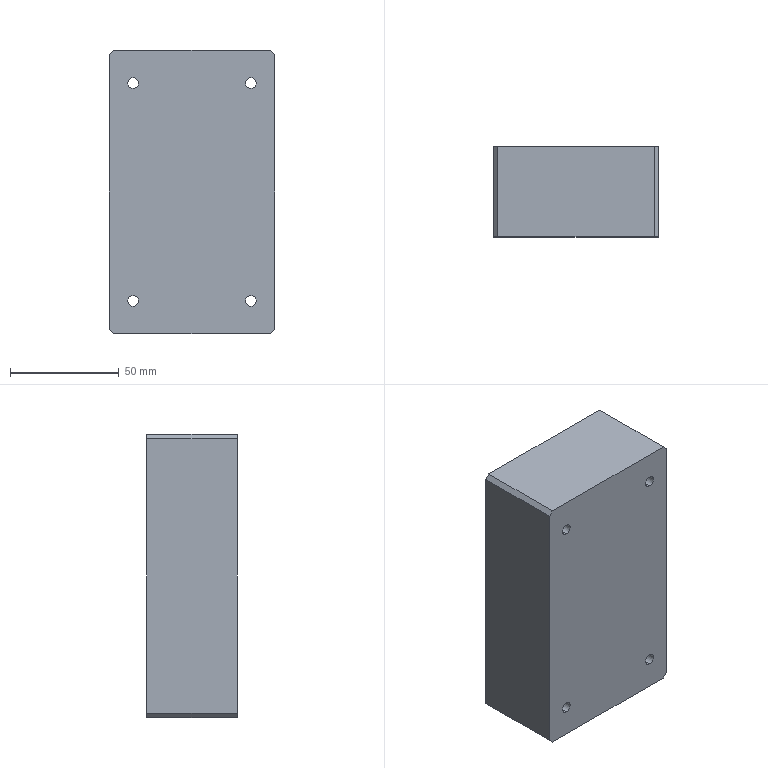Part | SolidWorks | features Chamfer 1, Extrusion 1, HoleWzd 1 | 1 solid | 18 faces | box 76 x 41.5 x 130 mm | volume 406429 mm3 | plane 10 | cylinder 8 | commonest cylinder face diameters 5 x8
STEP:
#1=CARTESIAN_POINT('',(-27.,-20.75,47.5));
#2=VERTEX_POINT('',#1);
#3=CARTESIAN_POINT('',(-27.,-20.75,52.5));
#4=VERTEX_POINT('',#3);
#5=CARTESIAN_POINT('',(-27.,-20.75,50.));
#6=DIRECTION('',(0.,1.,0.));
#7=DIRECTION('',(0.,0.,1.));
#8=AXIS2_PLACEMENT_3D('',#5,#6,#7);
#9=CIRCLE('',#8,2.5);
#10=EDGE_CURVE('',#2,#4,#9,.T.);
#11=ORIENTED_EDGE('',*,*,#10,.F.);
#12=CARTESIAN_POINT('',(-27.,20.75,47.5));
#13=VERTEX_POINT('',#12);
#14=CARTESIAN_POINT('',(-27.,20.75,47.5));
#15=DIRECTION('',(0.,1.,0.));
#16=VECTOR('',#15,1000.);
#17=LINE('',#14,#16);
#18=EDGE_CURVE('',#2,#13,#17,.T.);
#19=ORIENTED_EDGE('',*,*,#18,.T.);
#20=CARTESIAN_POINT('',(-27.,20.75,52.5));
#21=VERTEX_POINT('',#20);
#22=CARTESIAN_POINT('',(-27.,20.75,50.));
#23=DIRECTION('',(0.,1.,0.));
#24=DIRECTION('',(0.,0.,1.));
#25=AXIS2_PLACEMENT_3D('',#22,#23,#24);
#26=CIRCLE('',#25,2.5);
#27=EDGE_CURVE('',#13,#21,#26,.T.);
#28=ORIENTED_EDGE('',*,*,#27,.T.);
#29=CARTESIAN_POINT('',(-27.,20.75,52.5));
#30=DIRECTION('',(0.,1.,0.));
#31=VECTOR('',#30,1000.);
#32=LINE('',#29,#31);
#33=EDGE_CURVE('',#4,#21,#32,.T.);
#34=ORIENTED_EDGE('',*,*,#33,.F.);
#35=EDGE_LOOP('',(#11,#19,#28,#34));
#36=FACE_OUTER_BOUND('',#35,.T.);
#37=CARTESIAN_POINT('',(-27.,20.75,50.));
#38=DIRECTION('',(0.,1.,0.));
#39=DIRECTION('',(0.,0.,1.));
#40=AXIS2_PLACEMENT_3D('',#37,#38,#39);
#41=CYLINDRICAL_SURFACE('',#40,2.5);
#42=ADVANCED_FACE('',(#36),#41,.F.);
#43=CARTESIAN_POINT('',(27.,-20.75,47.5));
#44=VERTEX_POINT('',#43);
#45=CARTESIAN_POINT('',(27.,-20.75,52.5));
#46=VERTEX_POINT('',#45);
#47=CARTESIAN_POINT('',(27.,-20.75,50.));
#48=DIRECTION('',(0.,1.,0.));
#49=DIRECTION('',(0.,0.,1.));
#50=AXIS2_PLACEMENT_3D('',#47,#48,#49);
#51=CIRCLE('',#50,2.5);
#52=EDGE_CURVE('',#44,#46,#51,.T.);
#53=ORIENTED_EDGE('',*,*,#52,.F.);
#54=CARTESIAN_POINT('',(27.,20.75,47.5));
#55=VERTEX_POINT('',#54);
#56=CARTESIAN_POINT('',(27.,20.75,47.5));
#57=DIRECTION('',(0.,1.,0.));
#58=VECTOR('',#57,1000.);
#59=LINE('',#56,#58);
#60=EDGE_CURVE('',#44,#55,#59,.T.);
#61=ORIENTED_EDGE('',*,*,#60,.T.);
#62=CARTESIAN_POINT('',(27.,20.75,52.5));
#63=VERTEX_POINT('',#62);
#64=CARTESIAN_POINT('',(27.,20.75,50.));
#65=DIRECTION('',(0.,1.,0.));
#66=DIRECTION('',(0.,0.,1.));
#67=AXIS2_PLACEMENT_3D('',#64,#65,#66);
#68=CIRCLE('',#67,2.5);
#69=EDGE_CURVE('',#55,#63,#68,.T.);
#70=ORIENTED_EDGE('',*,*,#69,.T.);
#71=CARTESIAN_POINT('',(27.,20.75,52.5));
#72=DIRECTION('',(0.,1.,0.));
#73=VECTOR('',#72,1000.);
#74=LINE('',#71,#73);
#75=EDGE_CURVE('',#46,#63,#74,.T.);
#76=ORIENTED_EDGE('',*,*,#75,.F.);
#77=EDGE_LOOP('',(#53,#61,#70,#76));
#78=FACE_OUTER_BOUND('',#77,.T.);
#79=CARTESIAN_POINT('',(27.,20.75,50.));
#80=DIRECTION('',(0.,1.,0.));
#81=DIRECTION('',(0.,0.,1.));
#82=AXIS2_PLACEMENT_3D('',#79,#80,#81);
#83=CYLINDRICAL_SURFACE('',#82,2.5);
#84=ADVANCED_FACE('',(#78),#83,.F.);
#85=CARTESIAN_POINT('',(27.,-20.75,-52.5));
#86=VERTEX_POINT('',#85);
#87=CARTESIAN_POINT('',(27.,-20.75,-47.5));
#88=VERTEX_POINT('',#87);
#89=CARTESIAN_POINT('',(27.,-20.75,-50.));
#90=DIRECTION('',(0.,1.,0.));
#91=DIRECTION('',(0.,0.,1.));
#92=AXIS2_PLACEMENT_3D('',#89,#90,#91);
#93=CIRCLE('',#92,2.5);
#94=EDGE_CURVE('',#86,#88,#93,.T.);
#95=ORIENTED_EDGE('',*,*,#94,.F.);
#96=CARTESIAN_POINT('',(27.,20.75,-52.5));
#97=VERTEX_POINT('',#96);
#98=CARTESIAN_POINT('',(27.,20.75,-52.5));
#99=DIRECTION('',(0.,1.,0.));
#100=VECTOR('',#99,1000.);
#101=LINE('',#98,#100);
#102=EDGE_CURVE('',#86,#97,#101,.T.);
#103=ORIENTED_EDGE('',*,*,#102,.T.);
#104=CARTESIAN_POINT('',(27.,20.75,-47.5));
#105=VERTEX_POINT('',#104);
#106=CARTESIAN_POINT('',(27.,20.75,-50.));
#107=DIRECTION('',(0.,1.,0.));
#108=DIRECTION('',(0.,0.,1.));
#109=AXIS2_PLACEMENT_3D('',#106,#107,#108);
#110=CIRCLE('',#109,2.5);
#111=EDGE_CURVE('',#97,#105,#110,.T.);
#112=ORIENTED_EDGE('',*,*,#111,.T.);
#113=CARTESIAN_POINT('',(27.,20.75,-47.5));
#114=DIRECTION('',(0.,1.,0.));
#115=VECTOR('',#114,1000.);
#116=LINE('',#113,#115);
#117=EDGE_CURVE('',#88,#105,#116,.T.);
#118=ORIENTED_EDGE('',*,*,#117,.F.);
#119=EDGE_LOOP('',(#95,#103,#112,#118));
#120=FACE_OUTER_BOUND('',#119,.T.);
#121=CARTESIAN_POINT('',(27.,20.75,-50.));
#122=DIRECTION('',(0.,1.,0.));
#123=DIRECTION('',(0.,0.,1.));
#124=AXIS2_PLACEMENT_3D('',#121,#122,#123);
#125=CYLINDRICAL_SURFACE('',#124,2.5);
#126=ADVANCED_FACE('',(#120),#125,.F.);
#127=CARTESIAN_POINT('',(-27.,-20.75,-52.5));
#128=VERTEX_POINT('',#127);
#129=CARTESIAN_POINT('',(-27.,-20.75,-47.5));
#130=VERTEX_POINT('',#129);
#131=CARTESIAN_POINT('',(-27.,-20.75,-50.));
#132=DIRECTION('',(0.,1.,0.));
#133=DIRECTION('',(0.,0.,1.));
#134=AXIS2_PLACEMENT_3D('',#131,#132,#133);
#135=CIRCLE('',#134,2.5);
#136=EDGE_CURVE('',#128,#130,#135,.T.);
#137=ORIENTED_EDGE('',*,*,#136,.F.);
#138=CARTESIAN_POINT('',(-27.,20.75,-52.5));
#139=VERTEX_POINT('',#138);
#140=CARTESIAN_POINT('',(-27.,20.75,-52.5));
#141=DIRECTION('',(0.,1.,0.));
#142=VECTOR('',#141,1000.);
#143=LINE('',#140,#142);
#144=EDGE_CURVE('',#128,#139,#143,.T.);
#145=ORIENTED_EDGE('',*,*,#144,.T.);
#146=CARTESIAN_POINT('',(-27.,20.75,-47.5));
#147=VERTEX_POINT('',#146);
#148=CARTESIAN_POINT('',(-27.,20.75,-50.));
#149=DIRECTION('',(0.,1.,0.));
#150=DIRECTION('',(0.,0.,1.));
#151=AXIS2_PLACEMENT_3D('',#148,#149,#150);
#152=CIRCLE('',#151,2.5);
#153=EDGE_CURVE('',#139,#147,#152,.T.);
#154=ORIENTED_EDGE('',*,*,#153,.T.);
#155=CARTESIAN_POINT('',(-27.,20.75,-47.5));
#156=DIRECTION('',(0.,1.,0.));
#157=VECTOR('',#156,1000.);
#158=LINE('',#155,#157);
#159=EDGE_CURVE('',#130,#147,#158,.T.);
#160=ORIENTED_EDGE('',*,*,#159,.F.);
#161=EDGE_LOOP('',(#137,#145,#154,#160));
#162=FACE_OUTER_BOUND('',#161,.T.);
#163=CARTESIAN_POINT('',(-27.,20.75,-50.));
#164=DIRECTION('',(0.,1.,0.));
#165=DIRECTION('',(0.,0.,1.));
#166=AXIS2_PLACEMENT_3D('',#163,#164,#165);
#167=CYLINDRICAL_SURFACE('',#166,2.5);
#168=ADVANCED_FACE('',(#162),#167,.F.);
#169=CARTESIAN_POINT('',(38.,20.75,63.));
#170=VERTEX_POINT('',#169);
#171=CARTESIAN_POINT('',(38.,20.75,-63.));
#172=VERTEX_POINT('',#171);
#173=CARTESIAN_POINT('',(38.,20.75,65.));
#174=DIRECTION('',(0.,0.,-1.));
#175=VECTOR('',#174,1000.);
#176=LINE('',#173,#175);
#177=EDGE_CURVE('',#170,#172,#176,.T.);
#178=ORIENTED_EDGE('',*,*,#177,.F.);
#179=CARTESIAN_POINT('',(38.,-20.75,63.));
#180=VERTEX_POINT('',#179);
#181=CARTESIAN_POINT('',(38.,-20.75,63.));
#182=DIRECTION('',(0.,-1.,0.));
#183=VECTOR('',#182,1000.);
#184=LINE('',#181,#183);
#185=EDGE_CURVE('',#170,#180,#184,.T.);
#186=ORIENTED_EDGE('',*,*,#185,.T.);
#187=CARTESIAN_POINT('',(38.,-20.75,-63.));
#188=VERTEX_POINT('',#187);
#189=CARTESIAN_POINT('',(38.,-20.75,65.));
#190=DIRECTION('',(0.,0.,-1.));
#191=VECTOR('',#190,1000.);
#192=LINE('',#189,#191);
#193=EDGE_CURVE('',#180,#188,#192,.T.);
#194=ORIENTED_EDGE('',*,*,#193,.T.);
#195=CARTESIAN_POINT('',(38.,20.75,-63.));
#196=DIRECTION('',(0.,1.,0.));
#197=VECTOR('',#196,1000.);
#198=LINE('',#195,#197);
#199=EDGE_CURVE('',#188,#172,#198,.T.);
#200=ORIENTED_EDGE('',*,*,#199,.T.);
#201=EDGE_LOOP('',(#178,#186,#194,#200));
#202=FACE_OUTER_BOUND('',#201,.T.);
#203=CARTESIAN_POINT('',(38.,20.75,65.));
#204=DIRECTION('',(-1.,0.,0.));
#205=DIRECTION('',(0.,0.,1.));
#206=AXIS2_PLACEMENT_3D('',#203,#204,#205);
#207=PLANE('',#206);
#208=ADVANCED_FACE('',(#202),#207,.F.);
#209=CARTESIAN_POINT('',(-27.,20.75,50.));
#210=DIRECTION('',(0.,1.,0.));
#211=DIRECTION('',(0.,0.,1.));
#212=AXIS2_PLACEMENT_3D('',#209,#210,#211);
#213=CIRCLE('',#212,2.5);
#214=EDGE_CURVE('',#21,#13,#213,.T.);
#215=ORIENTED_EDGE('',*,*,#214,.F.);
#216=ORIENTED_EDGE('',*,*,#27,.F.);
#217=EDGE_LOOP('',(#215,#216));
#218=FACE_BOUND('',#217,.T.);
#219=CARTESIAN_POINT('',(27.,20.75,50.));
#220=DIRECTION('',(0.,1.,0.));
#221=DIRECTION('',(0.,0.,1.));
#222=AXIS2_PLACEMENT_3D('',#219,#220,#221);
#223=CIRCLE('',#222,2.5);
#224=EDGE_CURVE('',#63,#55,#223,.T.);
#225=ORIENTED_EDGE('',*,*,#224,.F.);
#226=ORIENTED_EDGE('',*,*,#69,.F.);
#227=EDGE_LOOP('',(#225,#226));
#228=FACE_BOUND('',#227,.T.);
#229=CARTESIAN_POINT('',(27.,20.75,-50.));
#230=DIRECTION('',(0.,1.,0.));
#231=DIRECTION('',(0.,0.,1.));
#232=AXIS2_PLACEMENT_3D('',#229,#230,#231);
#233=CIRCLE('',#232,2.5);
#234=EDGE_CURVE('',#105,#97,#233,.T.);
#235=ORIENTED_EDGE('',*,*,#234,.F.);
#236=ORIENTED_EDGE('',*,*,#111,.F.);
#237=EDGE_LOOP('',(#235,#236));
#238=FACE_BOUND('',#237,.T.);
#239=CARTESIAN_POINT('',(-27.,20.75,-50.));
#240=DIRECTION('',(0.,1.,0.));
#241=DIRECTION('',(0.,0.,1.));
#242=AXIS2_PLACEMENT_3D('',#239,#240,#241);
#243=CIRCLE('',#242,2.5);
#244=EDGE_CURVE('',#147,#139,#243,.T.);
#245=ORIENTED_EDGE('',*,*,#244,.F.);
#246=ORIENTED_EDGE('',*,*,#153,.F.);
#247=EDGE_LOOP('',(#245,#246));
#248=FACE_BOUND('',#247,.T.);
#249=CARTESIAN_POINT('',(-38.,20.75,63.));
#250=VERTEX_POINT('',#249);
#251=CARTESIAN_POINT('',(-38.,20.75,-63.));
#252=VERTEX_POINT('',#251);
#253=CARTESIAN_POINT('',(-38.,20.75,65.));
#254=DIRECTION('',(0.,0.,-1.));
#255=VECTOR('',#254,1000.);
#256=LINE('',#253,#255);
#257=EDGE_CURVE('',#250,#252,#256,.T.);
#258=ORIENTED_EDGE('',*,*,#257,.F.);
#259=CARTESIAN_POINT('',(-36.,20.75,65.));
#260=VERTEX_POINT('',#259);
#261=CARTESIAN_POINT('',(-36.,20.75,65.));
#262=DIRECTION('',(0.7071,0.,0.7071));
#263=VECTOR('',#262,1000.);
#264=LINE('',#261,#263);
#265=EDGE_CURVE('',#250,#260,#264,.T.);
#266=ORIENTED_EDGE('',*,*,#265,.T.);
#267=CARTESIAN_POINT('',(36.,20.75,65.));
#268=VERTEX_POINT('',#267);
#269=CARTESIAN_POINT('',(-38.,20.75,65.));
#270=DIRECTION('',(-1.,0.,0.));
#271=VECTOR('',#270,1000.);
#272=LINE('',#269,#271);
#273=EDGE_CURVE('',#268,#260,#272,.T.);
#274=ORIENTED_EDGE('',*,*,#273,.F.);
#275=CARTESIAN_POINT('',(36.,20.75,65.));
#276=DIRECTION('',(0.7071,0.,-0.7071));
#277=VECTOR('',#276,1000.);
#278=LINE('',#275,#277);
#279=EDGE_CURVE('',#268,#170,#278,.T.);
#280=ORIENTED_EDGE('',*,*,#279,.T.);
#281=ORIENTED_EDGE('',*,*,#177,.T.);
#282=CARTESIAN_POINT('',(36.,20.75,-65.));
#283=VERTEX_POINT('',#282);
#284=CARTESIAN_POINT('',(38.,20.75,-63.));
#285=DIRECTION('',(-0.7071,0.,-0.7071));
#286=VECTOR('',#285,1000.);
#287=LINE('',#284,#286);
#288=EDGE_CURVE('',#172,#283,#287,.T.);
#289=ORIENTED_EDGE('',*,*,#288,.T.);
#290=CARTESIAN_POINT('',(-36.,20.75,-65.));
#291=VERTEX_POINT('',#290);
#292=CARTESIAN_POINT('',(-38.,20.75,-65.));
#293=DIRECTION('',(-1.,0.,0.));
#294=VECTOR('',#293,1000.);
#295=LINE('',#292,#294);
#296=EDGE_CURVE('',#283,#291,#295,.T.);
#297=ORIENTED_EDGE('',*,*,#296,.T.);
#298=CARTESIAN_POINT('',(-38.,20.75,-63.));
#299=DIRECTION('',(-0.7071,0.,0.7071));
#300=VECTOR('',#299,1000.);
#301=LINE('',#298,#300);
#302=EDGE_CURVE('',#291,#252,#301,.T.);
#303=ORIENTED_EDGE('',*,*,#302,.T.);
#304=EDGE_LOOP('',(#258,#266,#274,#280,#281,#289,#297,#303));
#305=FACE_OUTER_BOUND('',#304,.T.);
#306=CARTESIAN_POINT('',(-38.,20.75,65.));
#307=DIRECTION('',(0.,-1.,0.));
#308=DIRECTION('',(0.,0.,-1.));
#309=AXIS2_PLACEMENT_3D('',#306,#307,#308);
#310=PLANE('',#309);
#311=ADVANCED_FACE('',(#218,#228,#238,#248,#305),#310,.F.);
#312=CARTESIAN_POINT('',(-38.,-20.75,63.));
#313=VERTEX_POINT('',#312);
#314=CARTESIAN_POINT('',(-38.,-20.75,-63.));
#315=VERTEX_POINT('',#314);
#316=CARTESIAN_POINT('',(-38.,-20.75,65.));
#317=DIRECTION('',(0.,0.,-1.));
#318=VECTOR('',#317,1000.);
#319=LINE('',#316,#318);
#320=EDGE_CURVE('',#313,#315,#319,.T.);
#321=ORIENTED_EDGE('',*,*,#320,.F.);
#322=CARTESIAN_POINT('',(-38.,20.75,63.));
#323=DIRECTION('',(0.,1.,0.));
#324=VECTOR('',#323,1000.);
#325=LINE('',#322,#324);
#326=EDGE_CURVE('',#313,#250,#325,.T.);
#327=ORIENTED_EDGE('',*,*,#326,.T.);
#328=ORIENTED_EDGE('',*,*,#257,.T.);
#329=CARTESIAN_POINT('',(-38.,20.75,-63.));
#330=DIRECTION('',(0.,-1.,0.));
#331=VECTOR('',#330,1000.);
#332=LINE('',#329,#331);
#333=EDGE_CURVE('',#252,#315,#332,.T.);
#334=ORIENTED_EDGE('',*,*,#333,.T.);
#335=EDGE_LOOP('',(#321,#327,#328,#334));
#336=FACE_OUTER_BOUND('',#335,.T.);
#337=CARTESIAN_POINT('',(-38.,20.75,65.));
#338=DIRECTION('',(1.,0.,0.));
#339=DIRECTION('',(0.,1.,0.));
#340=AXIS2_PLACEMENT_3D('',#337,#338,#339);
#341=PLANE('',#340);
#342=ADVANCED_FACE('',(#336),#341,.F.);
#343=CARTESIAN_POINT('',(-27.,-20.75,50.));
#344=DIRECTION('',(0.,1.,0.));
#345=DIRECTION('',(0.,0.,1.));
#346=AXIS2_PLACEMENT_3D('',#343,#344,#345);
#347=CIRCLE('',#346,2.5);
#348=EDGE_CURVE('',#4,#2,#347,.T.);
#349=ORIENTED_EDGE('',*,*,#348,.T.);
#350=ORIENTED_EDGE('',*,*,#10,.T.);
#351=EDGE_LOOP('',(#349,#350));
#352=FACE_BOUND('',#351,.T.);
#353=CARTESIAN_POINT('',(27.,-20.75,50.));
#354=DIRECTION('',(0.,1.,0.));
#355=DIRECTION('',(0.,0.,1.));
#356=AXIS2_PLACEMENT_3D('',#353,#354,#355);
#357=CIRCLE('',#356,2.5);
#358=EDGE_CURVE('',#46,#44,#357,.T.);
#359=ORIENTED_EDGE('',*,*,#358,.T.);
#360=ORIENTED_EDGE('',*,*,#52,.T.);
#361=EDGE_LOOP('',(#359,#360));
#362=FACE_BOUND('',#361,.T.);
#363=CARTESIAN_POINT('',(27.,-20.75,-50.));
#364=DIRECTION('',(0.,1.,0.));
#365=DIRECTION('',(0.,0.,1.));
#366=AXIS2_PLACEMENT_3D('',#363,#364,#365);
#367=CIRCLE('',#366,2.5);
#368=EDGE_CURVE('',#88,#86,#367,.T.);
#369=ORIENTED_EDGE('',*,*,#368,.T.);
#370=ORIENTED_EDGE('',*,*,#94,.T.);
#371=EDGE_LOOP('',(#369,#370));
#372=FACE_BOUND('',#371,.T.);
#373=CARTESIAN_POINT('',(-27.,-20.75,-50.));
#374=DIRECTION('',(0.,1.,0.));
#375=DIRECTION('',(0.,0.,1.));
#376=AXIS2_PLACEMENT_3D('',#373,#374,#375);
#377=CIRCLE('',#376,2.5);
#378=EDGE_CURVE('',#130,#128,#377,.T.);
#379=ORIENTED_EDGE('',*,*,#378,.T.);
#380=ORIENTED_EDGE('',*,*,#136,.T.);
#381=EDGE_LOOP('',(#379,#380));
#382=FACE_BOUND('',#381,.T.);
#383=CARTESIAN_POINT('',(-36.,-20.75,65.));
#384=VERTEX_POINT('',#383);
#385=CARTESIAN_POINT('',(36.,-20.75,65.));
#386=VERTEX_POINT('',#385);
#387=CARTESIAN_POINT('',(-38.,-20.75,65.));
#388=DIRECTION('',(1.,0.,0.));
#389=VECTOR('',#388,1000.);
#390=LINE('',#387,#389);
#391=EDGE_CURVE('',#384,#386,#390,.T.);
#392=ORIENTED_EDGE('',*,*,#391,.F.);
#393=CARTESIAN_POINT('',(-36.,-20.75,65.));
#394=DIRECTION('',(-0.7071,0.,-0.7071));
#395=VECTOR('',#394,1000.);
#396=LINE('',#393,#395);
#397=EDGE_CURVE('',#384,#313,#396,.T.);
#398=ORIENTED_EDGE('',*,*,#397,.T.);
#399=ORIENTED_EDGE('',*,*,#320,.T.);
#400=CARTESIAN_POINT('',(-36.,-20.75,-65.));
#401=VERTEX_POINT('',#400);
#402=CARTESIAN_POINT('',(-38.,-20.75,-63.));
#403=DIRECTION('',(0.7071,0.,-0.7071));
#404=VECTOR('',#403,1000.);
#405=LINE('',#402,#404);
#406=EDGE_CURVE('',#315,#401,#405,.T.);
#407=ORIENTED_EDGE('',*,*,#406,.T.);
#408=CARTESIAN_POINT('',(36.,-20.75,-65.));
#409=VERTEX_POINT('',#408);
#410=CARTESIAN_POINT('',(-38.,-20.75,-65.));
#411=DIRECTION('',(1.,0.,0.));
#412=VECTOR('',#411,1000.);
#413=LINE('',#410,#412);
#414=EDGE_CURVE('',#401,#409,#413,.T.);
#415=ORIENTED_EDGE('',*,*,#414,.T.);
#416=CARTESIAN_POINT('',(38.,-20.75,-63.));
#417=DIRECTION('',(0.7071,0.,0.7071));
#418=VECTOR('',#417,1000.);
#419=LINE('',#416,#418);
#420=EDGE_CURVE('',#409,#188,#419,.T.);
#421=ORIENTED_EDGE('',*,*,#420,.T.);
#422=ORIENTED_EDGE('',*,*,#193,.F.);
#423=CARTESIAN_POINT('',(36.,-20.75,65.));
#424=DIRECTION('',(-0.7071,0.,0.7071));
#425=VECTOR('',#424,1000.);
#426=LINE('',#423,#425);
#427=EDGE_CURVE('',#180,#386,#426,.T.);
#428=ORIENTED_EDGE('',*,*,#427,.T.);
#429=EDGE_LOOP('',(#392,#398,#399,#407,#415,#421,#422,#428));
#430=FACE_OUTER_BOUND('',#429,.T.);
#431=CARTESIAN_POINT('',(-38.,-20.75,65.));
#432=DIRECTION('',(0.,1.,0.));
#433=DIRECTION('',(0.,0.,1.));
#434=AXIS2_PLACEMENT_3D('',#431,#432,#433);
#435=PLANE('',#434);
#436=ADVANCED_FACE('',(#352,#362,#372,#382,#430),#435,.F.);
#437=ORIENTED_EDGE('',*,*,#273,.T.);
#438=CARTESIAN_POINT('',(-36.,-20.75,65.));
#439=DIRECTION('',(0.,-1.,0.));
#440=VECTOR('',#439,1000.);
#441=LINE('',#438,#440);
#442=EDGE_CURVE('',#260,#384,#441,.T.);
#443=ORIENTED_EDGE('',*,*,#442,.T.);
#444=ORIENTED_EDGE('',*,*,#391,.T.);
#445=CARTESIAN_POINT('',(36.,20.75,65.));
#446=DIRECTION('',(0.,1.,0.));
#447=VECTOR('',#446,1000.);
#448=LINE('',#445,#447);
#449=EDGE_CURVE('',#386,#268,#448,.T.);
#450=ORIENTED_EDGE('',*,*,#449,.T.);
#451=EDGE_LOOP('',(#437,#443,#444,#450));
#452=FACE_OUTER_BOUND('',#451,.T.);
#453=CARTESIAN_POINT('',(0.,0.,65.));
#454=DIRECTION('',(0.,0.,1.));
#455=DIRECTION('',(1.,0.,0.));
#456=AXIS2_PLACEMENT_3D('',#453,#454,#455);
#457=PLANE('',#456);
#458=ADVANCED_FACE('',(#452),#457,.T.);
#459=ORIENTED_EDGE('',*,*,#414,.F.);
#460=CARTESIAN_POINT('',(-36.,0.,-65.));
#461=DIRECTION('',(0.,1.,0.));
#462=VECTOR('',#461,1000.);
#463=LINE('',#460,#462);
#464=EDGE_CURVE('',#401,#291,#463,.T.);
#465=ORIENTED_EDGE('',*,*,#464,.T.);
#466=ORIENTED_EDGE('',*,*,#296,.F.);
#467=CARTESIAN_POINT('',(36.,0.,-65.));
#468=DIRECTION('',(0.,-1.,0.));
#469=VECTOR('',#468,1000.);
#470=LINE('',#467,#469);
#471=EDGE_CURVE('',#283,#409,#470,.T.);
#472=ORIENTED_EDGE('',*,*,#471,.T.);
#473=EDGE_LOOP('',(#459,#465,#466,#472));
#474=FACE_OUTER_BOUND('',#473,.T.);
#475=CARTESIAN_POINT('',(0.,0.,-65.));
#476=DIRECTION('',(0.,0.,1.));
#477=DIRECTION('',(1.,0.,0.));
#478=AXIS2_PLACEMENT_3D('',#475,#476,#477);
#479=PLANE('',#478);
#480=ADVANCED_FACE('',(#474),#479,.F.);
#481=ORIENTED_EDGE('',*,*,#144,.F.);
#482=ORIENTED_EDGE('',*,*,#378,.F.);
#483=ORIENTED_EDGE('',*,*,#159,.T.);
#484=ORIENTED_EDGE('',*,*,#244,.T.);
#485=EDGE_LOOP('',(#481,#482,#483,#484));
#486=FACE_OUTER_BOUND('',#485,.T.);
#487=CARTESIAN_POINT('',(-27.,20.75,-50.));
#488=DIRECTION('',(0.,1.,0.));
#489=DIRECTION('',(0.,0.,1.));
#490=AXIS2_PLACEMENT_3D('',#487,#488,#489);
#491=CYLINDRICAL_SURFACE('',#490,2.5);
#492=ADVANCED_FACE('',(#486),#491,.F.);
#493=ORIENTED_EDGE('',*,*,#102,.F.);
#494=ORIENTED_EDGE('',*,*,#368,.F.);
#495=ORIENTED_EDGE('',*,*,#117,.T.);
#496=ORIENTED_EDGE('',*,*,#234,.T.);
#497=EDGE_LOOP('',(#493,#494,#495,#496));
#498=FACE_OUTER_BOUND('',#497,.T.);
#499=CARTESIAN_POINT('',(27.,20.75,-50.));
#500=DIRECTION('',(0.,1.,0.));
#501=DIRECTION('',(0.,0.,1.));
#502=AXIS2_PLACEMENT_3D('',#499,#500,#501);
#503=CYLINDRICAL_SURFACE('',#502,2.5);
#504=ADVANCED_FACE('',(#498),#503,.F.);
#505=ORIENTED_EDGE('',*,*,#60,.F.);
#506=ORIENTED_EDGE('',*,*,#358,.F.);
#507=ORIENTED_EDGE('',*,*,#75,.T.);
#508=ORIENTED_EDGE('',*,*,#224,.T.);
#509=EDGE_LOOP('',(#505,#506,#507,#508));
#510=FACE_OUTER_BOUND('',#509,.T.);
#511=CARTESIAN_POINT('',(27.,20.75,50.));
#512=DIRECTION('',(0.,1.,0.));
#513=DIRECTION('',(0.,0.,1.));
#514=AXIS2_PLACEMENT_3D('',#511,#512,#513);
#515=CYLINDRICAL_SURFACE('',#514,2.5);
#516=ADVANCED_FACE('',(#510),#515,.F.);
#517=ORIENTED_EDGE('',*,*,#18,.F.);
#518=ORIENTED_EDGE('',*,*,#348,.F.);
#519=ORIENTED_EDGE('',*,*,#33,.T.);
#520=ORIENTED_EDGE('',*,*,#214,.T.);
#521=EDGE_LOOP('',(#517,#518,#519,#520));
#522=FACE_OUTER_BOUND('',#521,.T.);
#523=CARTESIAN_POINT('',(-27.,20.75,50.));
#524=DIRECTION('',(0.,1.,0.));
#525=DIRECTION('',(0.,0.,1.));
#526=AXIS2_PLACEMENT_3D('',#523,#524,#525);
#527=CYLINDRICAL_SURFACE('',#526,2.5);
#528=ADVANCED_FACE('',(#522),#527,.F.);
#529=ORIENTED_EDGE('',*,*,#265,.F.);
#530=ORIENTED_EDGE('',*,*,#326,.F.);
#531=ORIENTED_EDGE('',*,*,#397,.F.);
#532=ORIENTED_EDGE('',*,*,#442,.F.);
#533=EDGE_LOOP('',(#529,#530,#531,#532));
#534=FACE_OUTER_BOUND('',#533,.T.);
#535=CARTESIAN_POINT('',(-36.,0.,65.));
#536=DIRECTION('',(-0.7071,0.,0.7071));
#537=DIRECTION('',(0.,1.,0.));
#538=AXIS2_PLACEMENT_3D('',#535,#536,#537);
#539=PLANE('',#538);
#540=ADVANCED_FACE('',(#534),#539,.T.);
#541=ORIENTED_EDGE('',*,*,#427,.F.);
#542=ORIENTED_EDGE('',*,*,#185,.F.);
#543=ORIENTED_EDGE('',*,*,#279,.F.);
#544=ORIENTED_EDGE('',*,*,#449,.F.);
#545=EDGE_LOOP('',(#541,#542,#543,#544));
#546=FACE_OUTER_BOUND('',#545,.T.);
#547=CARTESIAN_POINT('',(36.,0.,65.));
#548=DIRECTION('',(0.7071,0.,0.7071));
#549=DIRECTION('',(0.,-1.,0.));
#550=AXIS2_PLACEMENT_3D('',#547,#548,#549);
#551=PLANE('',#550);
#552=ADVANCED_FACE('',(#546),#551,.T.);
#553=ORIENTED_EDGE('',*,*,#302,.F.);
#554=ORIENTED_EDGE('',*,*,#464,.F.);
#555=ORIENTED_EDGE('',*,*,#406,.F.);
#556=ORIENTED_EDGE('',*,*,#333,.F.);
#557=EDGE_LOOP('',(#553,#554,#555,#556));
#558=FACE_OUTER_BOUND('',#557,.T.);
#559=CARTESIAN_POINT('',(-38.,20.75,-63.));
#560=DIRECTION('',(0.7071,0.,0.7071));
#561=DIRECTION('',(0.,-1.,0.));
#562=AXIS2_PLACEMENT_3D('',#559,#560,#561);
#563=PLANE('',#562);
#564=ADVANCED_FACE('',(#558),#563,.F.);
#565=ORIENTED_EDGE('',*,*,#420,.F.);
#566=ORIENTED_EDGE('',*,*,#471,.F.);
#567=ORIENTED_EDGE('',*,*,#288,.F.);
#568=ORIENTED_EDGE('',*,*,#199,.F.);
#569=EDGE_LOOP('',(#565,#566,#567,#568));
#570=FACE_OUTER_BOUND('',#569,.T.);
#571=CARTESIAN_POINT('',(38.,20.75,-63.));
#572=DIRECTION('',(-0.7071,0.,0.7071));
#573=DIRECTION('',(0.,1.,0.));
#574=AXIS2_PLACEMENT_3D('',#571,#572,#573);
#575=PLANE('',#574);
#576=ADVANCED_FACE('',(#570),#575,.F.);
#577=CLOSED_SHELL('',(#42,#84,#126,#168,#208,#311,#342,#436,#458,#480,#492,#504,#516,#528,#540,#552,#564,#576));
#578=MANIFOLD_SOLID_BREP('',#577);
#579=CARTESIAN_POINT('',(0.,0.,0.));
#580=DIRECTION('',(0.,0.,1.));
#581=DIRECTION('',(1.,0.,0.));
#582=AXIS2_PLACEMENT_3D('',#579,#580,#581);
#583=(LENGTH_UNIT()NAMED_UNIT(*)SI_UNIT(.MILLI.,.METRE.));
#584=UNCERTAINTY_MEASURE_WITH_UNIT(LENGTH_MEASURE(0.00001),#583,'','');
#585=(NAMED_UNIT(*)PLANE_ANGLE_UNIT()SI_UNIT($,.RADIAN.));
#586=(NAMED_UNIT(*)SI_UNIT($,.STERADIAN.)SOLID_ANGLE_UNIT());
#587=(GEOMETRIC_REPRESENTATION_CONTEXT(3)GLOBAL_UNCERTAINTY_ASSIGNED_CONTEXT((#584))GLOBAL_UNIT_ASSIGNED_CONTEXT((#583,#585,#586))REPRESENTATION_CONTEXT('',''));
#588=ADVANCED_BREP_SHAPE_REPRESENTATION('',(#578,#582),#587);